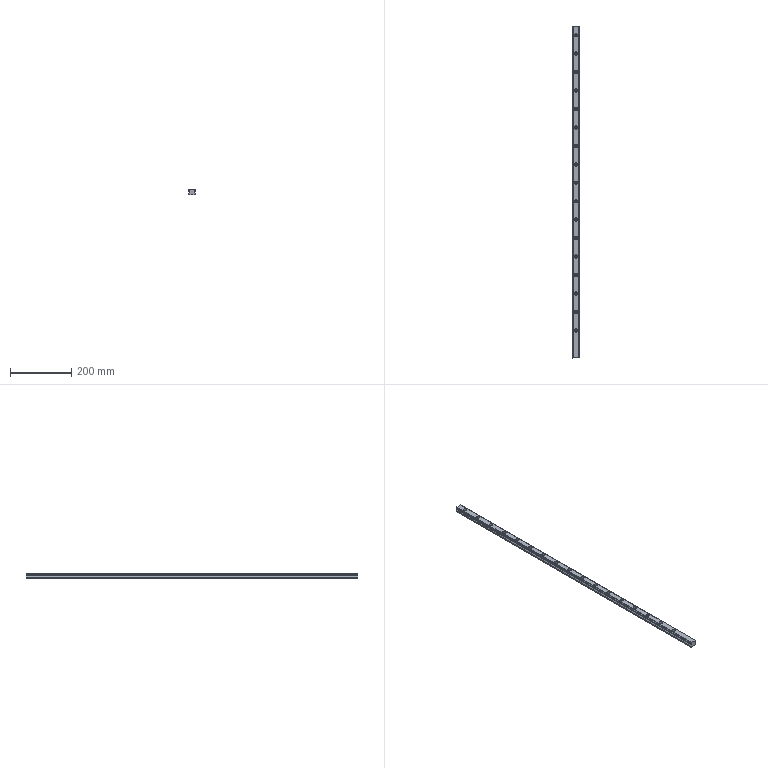Part | SolidWorks | features BaseBody 1 | 1 solid | 194 faces | box 23 x 1080 x 18 mm | volume 372740 mm3 | plane 110 | cylinder 76 | cone 8 | commonest cylinder face diameters 7 x34 11 x34 1 x4 4 x4